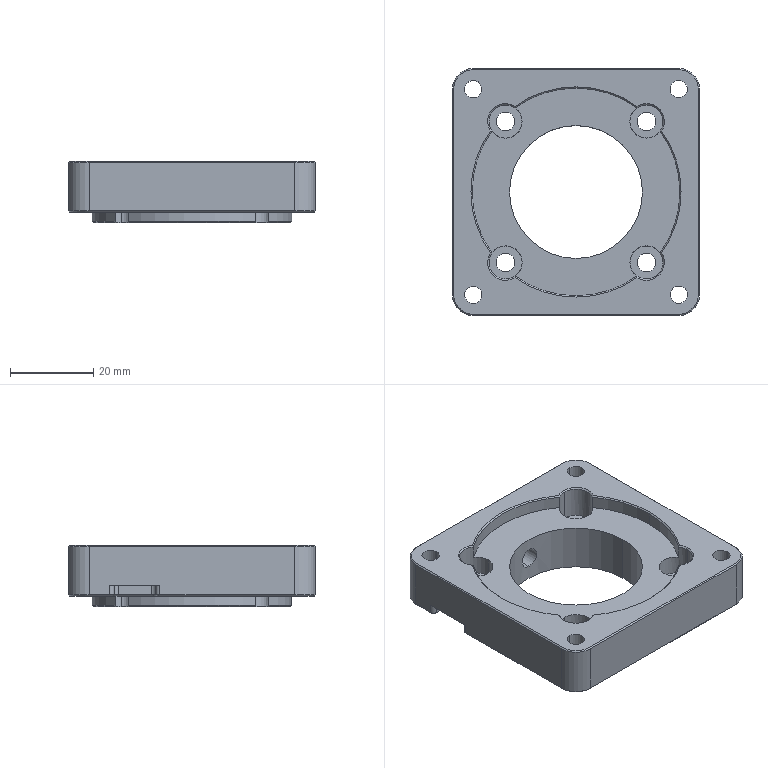Part | SolidWorks | features HoleWzd 3, ICE 3, CirPattern 2, Fillet 2, Chamfer 1, Cut 1, Extrusion 1, MirrorPattern 1 | 1 solid | 221 faces | box 59.5 x 59.5 x 14.7 mm | volume 28959 mm3 | plane 96 | cylinder 50 | spline 43 | cone 32 | commonest cylinder face diameters 2 x8 4.2 x8 4.5 x8 8 x8 48.1 x5 50 x5